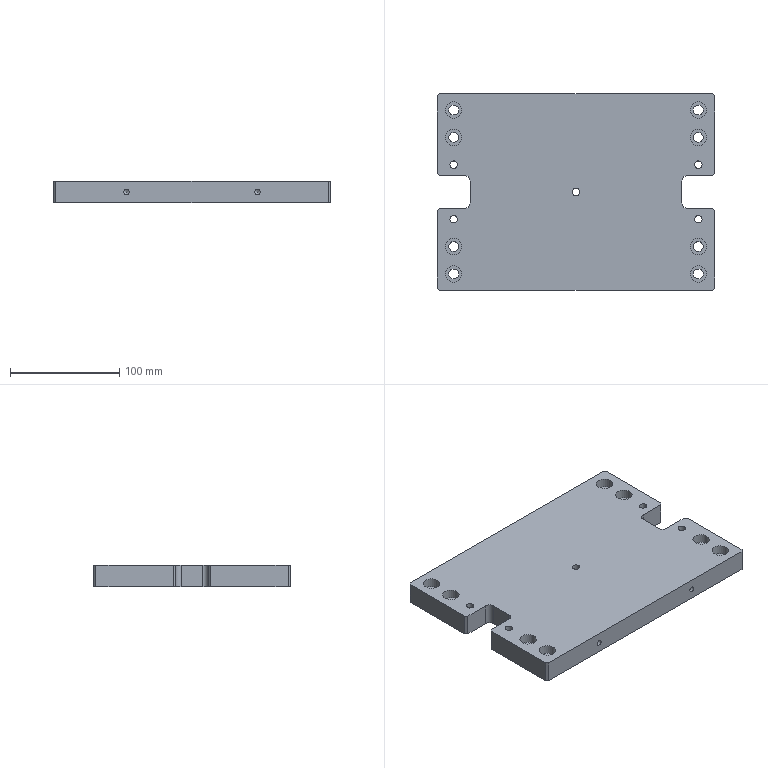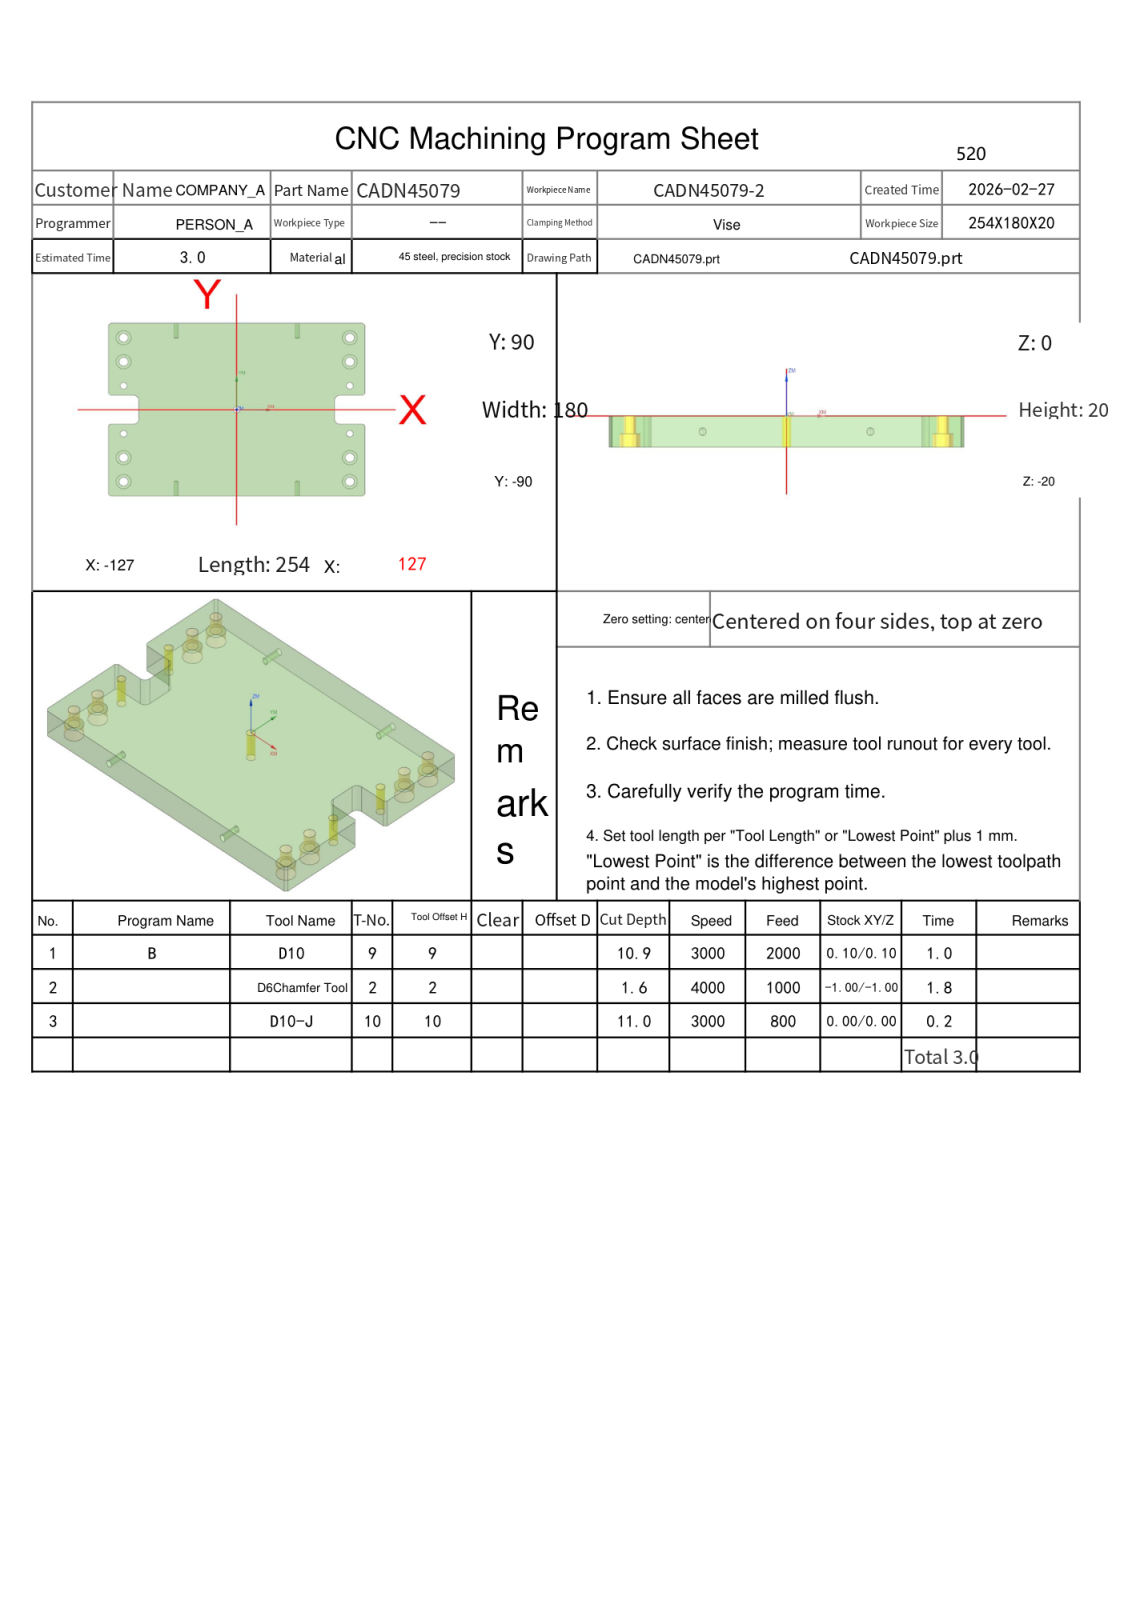NC program | NX | posted by the shop | part box 254 x 180 x 20 mm
Whole program:
%
O0001
(Machine time: 3.55 MIN)
(===Total Tool:3===)
(T9=D10     D=10.  R=0.   D-  H09 Z=-10.9 )
(T2=D6Chamfer Tool   D=6.   R=0.   D-  H02 Z=-1.6  )
(T10=D10-J  D=10.  R=0.   D-  H10 Z=-11.  )
G80 G90 G17 G49 G40
G91 G28 Z0
M01
N1 T09 M06
(D10  D=10. R=0. H=09 ce=0.10 di=0.10)
G00 G90 G54 X122.242 Y99.97 M03 S3000
G43 H09 Z30.
M08
Z-.5
G01 X128.606 Y93.606 F2000.
X130.606 Y91.606
X136.97 Y85.242
G00 Z-1.
G01 X130.606 Y91.606
X128.606 Y93.606
X122.242 Y99.97
G00 Z-1.5
G01 X128.606 Y93.606
X130.606 Y91.606
X136.97 Y85.242
G00 Z-2.
G01 X130.606 Y91.606
X128.606 Y93.606
X122.242 Y99.97
G00 Z-2.5
G01 X128.606 Y93.606
X130.606 Y91.606
X136.97 Y85.242
G00 Z-3.
G01 X130.606 Y91.606
X128.606 Y93.606
X122.242 Y99.97
G00 Z-3.5
G01 X128.606 Y93.606
X130.606 Y91.606
X136.97 Y85.242
G00 Z-4.
G01 X130.606 Y91.606
X128.606 Y93.606
X122.242 Y99.97
G00 Z-4.5
G01 X128.606 Y93.606
X130.606 Y91.606
X136.97 Y85.242
G00 Z-5.
G01 X130.606 Y91.606
X128.606 Y93.606
X122.242 Y99.97
G00 Z-5.5
G01 X128.606 Y93.606
X130.606 Y91.606
X136.97 Y85.242
G00 Z-6.
G01 X130.606 Y91.606
X128.606 Y93.606
X122.242 Y99.97
G00 Z-6.5
G01 X128.606 Y93.606
X130.606 Y91.606
X136.97 Y85.242
G00 Z-7.
G01 X130.606 Y91.606
X128.606 Y93.606
X122.242 Y99.97
G00 Z-7.5
G01 X128.606 Y93.606
X130.606 Y91.606
X136.97 Y85.242
G00 Z-8.
G01 X130.606 Y91.606
X128.606 Y93.606
X122.242 Y99.97
G00 Z-8.5
G01 X128.606 Y93.606
X130.606 Y91.606
X136.97 Y85.242
G00 Z-9.
G01 X130.606 Y91.606
X128.606 Y93.606
X122.242 Y99.97
G00 Z-9.5
G01 X128.606 Y93.606
X130.606 Y91.606
X136.97 Y85.242
G00 Z-10.
G01 X130.606 Y91.606
X128.606 Y93.606
X122.242 Y99.97
G00 Z-10.5
G01 X128.606 Y93.606
X130.606 Y91.606
X136.97 Y85.242
G00 Z-10.9
G01 X130.606 Y91.606
X128.606 Y93.606
X122.242 Y99.97
G00 Z30.
X136.97 Y-85.242
Z-.5
G01 X130.606 Y-91.606
X128.606 Y-93.606
X122.242 Y-99.97
G00 Z-1.
G01 X128.606 Y-93.606
X130.606 Y-91.606
X136.97 Y-85.242
G00 Z-1.5
G01 X130.606 Y-91.606
X128.606 Y-93.606
X122.242 Y-99.97
G00 Z-2.
G01 X128.606 Y-93.606
X130.606 Y-91.606
X136.97 Y-85.242
G00 Z-2.5
G01 X130.606 Y-91.606
X128.606 Y-93.606
X122.242 Y-99.97
G00 Z-3.
G01 X128.606 Y-93.606
X130.606 Y-91.606
X136.97 Y-85.242
G00 Z-3.5
G01 X130.606 Y-91.606
X128.606 Y-93.606
X122.242 Y-99.97
G00 Z-4.
G01 X128.606 Y-93.606
X130.606 Y-91.606
X136.97 Y-85.242
G00 Z-4.5
G01 X130.606 Y-91.606
X128.606 Y-93.606
X122.242 Y-99.97
G00 Z-5.
G01 X128.606 Y-93.606
X130.606 Y-91.606
X136.97 Y-85.242
G00 Z-5.5
G01 X130.606 Y-91.606
X128.606 Y-93.606
X122.242 Y-99.97
G00 Z-6.
G01 X128.606 Y-93.606
X130.606 Y-91.606
X136.97 Y-85.242
G00 Z-6.5
G01 X130.606 Y-91.606
X128.606 Y-93.606
X122.242 Y-99.97
G00 Z-7.
G01 X128.606 Y-93.606
X130.606 Y-91.606
X136.97 Y-85.242
G00 Z-7.5
G01 X130.606 Y-91.606
X128.606 Y-93.606
X122.242 Y-99.97
G00 Z-8.
G01 X128.606 Y-93.606
X130.606 Y-91.606
X136.97 Y-85.242
G00 Z-8.5
G01 X130.606 Y-91.606
X128.606 Y-93.606
X122.242 Y-99.97
G00 Z-9.
G01 X128.606 Y-93.606
X130.606 Y-91.606
X136.97 Y-85.242
G00 Z-9.5
G01 X130.606 Y-91.606
X128.606 Y-93.606
X122.242 Y-99.97
G00 Z-10.
G01 X128.606 Y-93.606
X130.606 Y-91.606
X136.97 Y-85.242
G00 Z-10.5
G01 X130.606 Y-91.606
X128.606 Y-93.606
X122.242 Y-99.97
G00 Z-10.9
G01 X128.606 Y-93.606
X130.606 Y-91.606
X136.97 Y-85.242
G00 Z30.
X-122.242 Y-99.97
Z-.5
G01 X-128.606 Y-93.606
X-130.606 Y-91.606
X-136.97 Y-85.242
G00 Z-1.
G01 X-130.606 Y-91.606
X-128.606 Y-93.606
X-122.242 Y-99.97
G00 Z-1.5
G01 X-128.606 Y-93.606
X-130.606 Y-91.606
X-136.97 Y-85.242
G00 Z-2.
G01 X-130.606 Y-91.606
X-128.606 Y-93.606
X-122.242 Y-99.97
G00 Z-2.5
G01 X-128.606 Y-93.606
X-130.606 Y-91.606
X-136.97 Y-85.242
G00 Z-3.
G01 X-130.606 Y-91.606
X-128.606 Y-93.606
X-122.242 Y-99.97
G00 Z-3.5
G01 X-128.606 Y-93.606
X-130.606 Y-91.606
X-136.97 Y-85.242
G00 Z-4.
G01 X-130.606 Y-91.606
X-128.606 Y-93.606
X-122.242 Y-99.97
G00 Z-4.5
G01 X-128.606 Y-93.606
X-130.606 Y-91.606
X-136.97 Y-85.242
G00 Z-5.
G01 X-130.606 Y-91.606
X-128.606 Y-93.606
X-122.242 Y-99.97
G00 Z-5.5
G01 X-128.606 Y-93.606
X-130.606 Y-91.606
X-136.97 Y-85.242
G00 Z-6.
G01 X-130.606 Y-91.606
X-128.606 Y-93.606
X-122.242 Y-99.97
G00 Z-6.5
G01 X-128.606 Y-93.606
X-130.606 Y-91.606
X-136.97 Y-85.242
G00 Z-7.
G01 X-130.606 Y-91.606
X-128.606 Y-93.606
X-122.242 Y-99.97
G00 Z-7.5
G01 X-128.606 Y-93.606
X-130.606 Y-91.606
X-136.97 Y-85.242
G00 Z-8.
G01 X-130.606 Y-91.606
X-128.606 Y-93.606
X-122.242 Y-99.97
G00 Z-8.5
G01 X-128.606 Y-93.606
X-130.606 Y-91.606
X-136.97 Y-85.242
G00 Z-9.
G01 X-130.606 Y-91.606
X-128.606 Y-93.606
X-122.242 Y-99.97
G00 Z-9.5
G01 X-128.606 Y-93.606
X-130.606 Y-91.606
X-136.97 Y-85.242
G00 Z-10.
G01 X-130.606 Y-91.606
X-128.606 Y-93.606
X-122.242 Y-99.97
G00 Z-10.5
G01 X-128.606 Y-93.606
X-130.606 Y-91.606
X-136.97 Y-85.242
G00 Z-10.9
G01 X-130.606 Y-91.606
X-128.606 Y-93.606
X-122.242 Y-99.97
G00 Z30.
X-136.97 Y85.242
Z-.5
G01 X-130.606 Y91.606
X-128.606 Y93.606
X-122.242 Y99.97
G00 Z-1.
G01 X-128.606 Y93.606
X-130.606 Y91.606
X-136.97 Y85.242
G00 Z-1.5
G01 X-130.606 Y91.606
X-128.606 Y93.606
X-122.242 Y99.97
G00 Z-2.
G01 X-128.606 Y93.606
X-130.606 Y91.606
X-136.97 Y85.242
G00 Z-2.5
G01 X-130.606 Y91.606
X-128.606 Y93.606
X-122.242 Y99.97
G00 Z-3.
G01 X-128.606 Y93.606
X-130.606 Y91.606
X-136.97 Y85.242
G00 Z-3.5
G01 X-130.606 Y91.606
X-128.606 Y93.606
X-122.242 Y99.97
G00 Z-4.
G01 X-128.606 Y93.606
X-130.606 Y91.606
X-136.97 Y85.242
G00 Z-4.5
G01 X-130.606 Y91.606
X-128.606 Y93.606
X-122.242 Y99.97
G00 Z-5.
G01 X-128.606 Y93.606
X-130.606 Y91.606
X-136.97 Y85.242
G00 Z-5.5
G01 X-130.606 Y91.606
X-128.606 Y93.606
X-122.242 Y99.97
G00 Z-6.
G01 X-128.606 Y93.606
X-130.606 Y91.606
X-136.97 Y85.242
G00 Z-6.5
G01 X-130.606 Y91.606
X-128.606 Y93.606
X-122.242 Y99.97
G00 Z-7.
G01 X-128.606 Y93.606
X-130.606 Y91.606
X-136.97 Y85.242
G00 Z-7.5
G01 X-130.606 Y91.606
X-128.606 Y93.606
X-122.242 Y99.97
G00 Z-8.
G01 X-128.606 Y93.606
X-130.606 Y91.606
X-136.97 Y85.242
G00 Z-8.5
G01 X-130.606 Y91.606
X-128.606 Y93.606
X-122.242 Y99.97
G00 Z-9.
G01 X-128.606 Y93.606
X-130.606 Y91.606
X-136.97 Y85.242
G00 Z-9.5
G01 X-130.606 Y91.606
X-128.606 Y93.606
X-122.242 Y99.97
G00 Z-10.
G01 X-128.606 Y93.606
X-130.606 Y91.606
X-136.97 Y85.242
G00 Z-10.5
G01 X-130.606 Y91.606
X-128.606 Y93.606
X-122.242 Y99.97
G00 Z-10.9
G01 X-128.606 Y93.606
X-130.606 Y91.606
X-136.97 Y85.242
G00 Z30.
G91 G28 Z0.0
M05
M09
G91 G28 Z0.0
M01
N2 T02 M06
(D6Chamfer Tool  D=6. R=0. H=02 ce=-1.00 di=-0.80)
G00 G90 G54 X111.005 Y26.5 M03 S4000
G43 H02 Z30.
M08
Z-1.1
G01 Z-1.6 F300.
X110.7
G03 X109.2 Y25. I0.0 J-1.5
X112. Y22.2 I2.8 J0.0
X114.8 Y25. I0.0 J2.8
X112. Y27.8 I-2.8 J0.0
X109.2 Y25. I0.0 J-2.8
X110.7 Y23.5 I1.5 J0.0
G01 X111.005
Z-1.1
G00 Z30.
Y-23.5
Z-1.1
G01 Z-1.6
X110.7
G03 X109.2 Y-25. I0.0 J-1.5
X112. Y-27.8 I2.8 J0.0
X114.8 Y-25. I0.0 J2.8
X112. Y-22.2 I-2.8 J0.0
X109.2 Y-25. I0.0 J-2.8
X110.7 Y-26.5 I1.5 J0.0
G01 X111.005
Z-1.1
G00 Z30.
X-.995 Y1.5
Z-1.1
G01 Z-1.6
X-1.3
G03 X-2.8 Y0.0 I0.0 J-1.5
X0.0 Y-2.8 I2.8 J0.0
X2.8 Y0.0 I0.0 J2.8
X0.0 Y2.8 I-2.8 J0.0
X-2.8 Y0.0 I0.0 J-2.8
X-1.3 Y-1.5 I1.5 J0.0
G01 X-.995
Z-1.1
G00 Z30.
X-112.995 Y-23.5
Z-1.1
G01 Z-1.6
X-113.3
G03 X-114.8 Y-25. I0.0 J-1.5
X-112. Y-27.8 I2.8 J0.0
X-109.2 Y-25. I0.0 J2.8
X-112. Y-22.2 I-2.8 J0.0
X-114.8 Y-25. I0.0 J-2.8
X-113.3 Y-26.5 I1.5 J0.0
G01 X-112.995
Z-1.1
G00 Z30.
Y26.5
Z-1.1
G01 Z-1.6
X-113.3
G03 X-114.8 Y25. I0.0 J-1.5
X-112. Y22.2 I2.8 J0.0
X-109.2 Y25. I0.0 J2.8
X-112. Y27.8 I-2.8 J0.0
X-114.8 Y25. I0.0 J-2.8
X-113.3 Y23.5 I1.5 J0.0
G01 X-112.995
Z-1.1
G00 Z30.
G00 G90 X-.386 Y91.227 M03 S3500
Z30.
Z.172
G01 Z-1.2 F1000.
G03 X-.1 Y91.027 I1.286 J1.532
G01 X-.054 Y90.997
X0.0 Y91.
X125.
X125.259 Y90.966
X125.5 Y90.866
X125.707 Y90.707
X127.707 Y88.707
X127.866 Y88.5
X127.966 Y88.259
X128. Y88.
Y17.
X127.966 Y16.741
X127.866 Y16.5
X127.707 Y16.293
X125.707 Y14.293
X125.5 Y14.134
X125.259 Y14.034
X125. Y14.
X102.
G03 X98. Y10. I0.0 J-4.
G01 Y-10.
G03 X102. Y-14. I4. J0.0
G01 X125.
X125.259 Y-14.034
X125.5 Y-14.134
X125.707 Y-14.293
X127.707 Y-16.293
X127.866 Y-16.5
X127.966 Y-16.741
X128. Y-17.
Y-88.
X127.966 Y-88.259
X127.866 Y-88.5
X127.707 Y-88.707
X125.707 Y-90.707
X125.5 Y-90.866
X125.259 Y-90.966
X125. Y-91.
X-125.
X-125.259 Y-90.966
X-125.5 Y-90.866
X-125.707 Y-90.707
X-127.707 Y-88.707
X-127.866 Y-88.5
X-127.966 Y-88.259
X-128. Y-88.
Y-17.
X-127.966 Y-16.741
X-127.866 Y-16.5
X-127.707 Y-16.293
X-125.707 Y-14.293
X-125.5 Y-14.134
X-125.259 Y-14.034
X-125. Y-14.
X-102.
G03 X-98. Y-10. I0.0 J4.
G01 Y10.
G03 X-102. Y14. I-4. J0.0
G01 X-125.
X-125.259 Y14.034
X-125.5 Y14.134
X-125.707 Y14.293
X-127.707 Y16.293
X-127.866 Y16.5
X-127.966 Y16.741
X-128. Y17.
Y88.
X-127.966 Y88.259
X-127.866 Y88.5
X-127.707 Y88.707
X-125.707 Y90.707
X-125.5 Y90.866
X-125.259 Y90.966
X-125. Y91.
X0.0
X.054 Y90.997
X.1 Y91.027
G03 X.386 Y91.227 I-1. J1.732
G01 Z.172
G00 Z10.
X108.697 Y75.401
Z.23
G01 Z-1.2
G03 X108.519 Y75.102 I1.624 J-1.167
G01 X108.493 Y75.054
X108.5 Y75.
G03 X112. Y71.5 I3.5 J0.0
X115.5 Y75. I0.0 J3.5
X112. Y78.5 I-3.5 J0.0
X108.5 Y75. I0.0 J-3.5
G01 X108.493 Y74.946
X108.519 Y74.898
G03 X108.697 Y74.599 I1.802 J.868
G01 Z.23
G00 Z10.
Y50.401
Z.23
G01 Z-1.2
G03 X108.519 Y50.102 I1.624 J-1.167
G01 X108.493 Y50.054
X108.5 Y50.
G03 X112. Y46.5 I3.5 J0.0
X115.5 Y50. I0.0 J3.5
X112. Y53.5 I-3.5 J0.0
X108.5 Y50. I0.0 J-3.5
G01 X108.493 Y49.946
X108.519 Y49.898
G03 X108.697 Y49.599 I1.802 J.868
G01 Z.23
G00 Z10.
X109.792 Y25.404
Z.252
G01 Z-1.2
G03 X109.618 Y25.102 I1.638 J-1.147
G01 X109.592 Y25.054
X109.6 Y25.
G03 X112. Y22.6 I2.4 J0.0
X114.4 Y25. I0.0 J2.4
X112. Y27.4 I-2.4 J0.0
X109.6 Y25. I0.0 J-2.4
G01 X109.592 Y24.946
X109.618 Y24.898
G03 X109.792 Y24.596 I1.813 J.845
G01 Z.252
G00 Z10.
Y-24.596
Z.252
G01 Z-1.2
G03 X109.618 Y-24.898 I1.638 J-1.147
G01 X109.592 Y-24.946
X109.6 Y-25.
G03 X112. Y-27.4 I2.4 J0.0
X114.4 Y-25. I0.0 J2.4
X112. Y-22.6 I-2.4 J0.0
X109.6 Y-25. I0.0 J-2.4
G01 X109.592 Y-25.054
X109.618 Y-25.102
G03 X109.792 Y-25.404 I1.813 J.845
G01 Z.252
G00 Z10.
X108.697 Y-49.599
Z.23
G01 Z-1.2
G03 X108.519 Y-49.898 I1.624 J-1.167
G01 X108.493 Y-49.946
X108.5 Y-50.
G03 X112. Y-53.5 I3.5 J0.0
X115.5 Y-50. I0.0 J3.5
X112. Y-46.5 I-3.5 J0.0
X108.5 Y-50. I0.0 J-3.5
G01 X108.493 Y-50.054
X108.519 Y-50.102
G03 X108.697 Y-50.401 I1.802 J.868
G01 Z.23
G00 Z10.
Y-74.599
Z.23
G01 Z-1.2
G03 X108.519 Y-74.898 I1.624 J-1.167
G01 X108.493 Y-74.946
X108.5 Y-75.
G03 X112. Y-78.5 I3.5 J0.0
X115.5 Y-75. I0.0 J3.5
X112. Y-71.5 I-3.5 J0.0
X108.5 Y-75. I0.0 J-3.5
G01 X108.493 Y-75.054
X108.519 Y-75.102
G03 X108.697 Y-75.401 I1.802 J.868
G01 Z.23
G00 Z10.
X-2.208 Y.404
Z.252
G01 Z-1.2
G03 X-2.382 Y.102 I1.638 J-1.147
G01 X-2.408 Y.054
X-2.4 Y0.0
G03 X0.0 Y-2.4 I2.4 J0.0
X2.4 Y0.0 I0.0 J2.4
X0.0 Y2.4 I-2.4 J0.0
X-2.4 Y0.0 I0.0 J-2.4
G01 X-2.408 Y-.054
X-2.382 Y-.102
G03 X-2.208 Y-.404 I1.813 J.845
G01 Z.252
G00 Z10.
X-115.303 Y75.401
Z.23
G01 Z-1.2
G03 X-115.481 Y75.102 I1.624 J-1.167
G01 X-115.507 Y75.054
X-115.5 Y75.
G03 X-112. Y71.5 I3.5 J0.0
X-108.5 Y75. I0.0 J3.5
X-112. Y78.5 I-3.5 J0.0
X-115.5 Y75. I0.0 J-3.5
G01 X-115.507 Y74.946
X-115.481 Y74.898
G03 X-115.303 Y74.599 I1.802 J.868
G01 Z.23
G00 Z10.
Y50.401
Z.23
G01 Z-1.2
G03 X-115.481 Y50.102 I1.624 J-1.167
G01 X-115.507 Y50.054
X-115.5 Y50.
G03 X-112. Y46.5 I3.5 J0.0
X-108.5 Y50. I0.0 J3.5
X-112. Y53.5 I-3.5 J0.0
X-115.5 Y50. I0.0 J-3.5
G01 X-115.507 Y49.946
X-115.481 Y49.898
G03 X-115.303 Y49.599 I1.802 J.868
G01 Z.23
G00 Z10.
X-114.208 Y25.404
Z.252
G01 Z-1.2
G03 X-114.382 Y25.102 I1.638 J-1.147
G01 X-114.408 Y25.054
X-114.4 Y25.
G03 X-112. Y22.6 I2.4 J0.0
X-109.6 Y25. I0.0 J2.4
X-112. Y27.4 I-2.4 J0.0
X-114.4 Y25. I0.0 J-2.4
G01 X-114.408 Y24.946
X-114.382 Y24.898
G03 X-114.208 Y24.596 I1.813 J.845
G01 Z.252
G00 Z10.
Y-24.596
Z.252
G01 Z-1.2
G03 X-114.382 Y-24.898 I1.638 J-1.147
G01 X-114.408 Y-24.946
X-114.4 Y-25.
G03 X-112. Y-27.4 I2.4 J0.0
X-109.6 Y-25. I0.0 J2.4
X-112. Y-22.6 I-2.4 J0.0
X-114.4 Y-25. I0.0 J-2.4
G01 X-114.408 Y-25.054
X-114.382 Y-25.102
G03 X-114.208 Y-25.404 I1.813 J.845
G01 Z.252
G00 Z10.
X-115.303 Y-49.599
Z.23
G01 Z-1.2
G03 X-115.481 Y-49.898 I1.624 J-1.167
G01 X-115.507 Y-49.946
X-115.5 Y-50.
G03 X-112. Y-53.5 I3.5 J0.0
X-108.5 Y-50. I0.0 J3.5
X-112. Y-46.5 I-3.5 J0.0
X-115.5 Y-50. I0.0 J-3.5
G01 X-115.507 Y-50.054
X-115.481 Y-50.102
G03 X-115.303 Y-50.401 I1.802 J.868
G01 Z.23
G00 Z10.
Y-74.599
Z.23
G01 Z-1.2
G03 X-115.481 Y-74.898 I1.624 J-1.167
G01 X-115.507 Y-74.946
X-115.5 Y-75.
G03 X-112. Y-78.5 I3.5 J0.0
X-108.5 Y-75. I0.0 J3.5
X-112. Y-71.5 I-3.5 J0.0
X-115.5 Y-75. I0.0 J-3.5
G01 X-115.507 Y-75.054
X-115.481 Y-75.102
G03 X-115.303 Y-75.401 I1.802 J.868
G01 Z.23
G00 Z30.
G91 G28 Z0.0
M05
M09
G91 G28 Z0.0
M01
N3 T10 M06
(D10-J  D=10. R=0. H=10 ce=0.00 di=0.00)
G00 G90 G54 X-124.293 Y-97.778 M03 S3000
G43 H10 Z30.
M08
Z-10.
G01 Z-11. F800.
X-128.536 Y-93.536
X-130.536 Y-91.536
X-134.778 Y-87.293
Z-10.
G00 Z30.
Y87.293
Z-10.
G01 Z-11.
X-130.536 Y91.536
X-128.536 Y93.536
X-124.293 Y97.778
Z-10.
G00 Z30.
X124.293
Z-10.
G01 Z-11.
X128.536 Y93.536
X130.536 Y91.536
X134.778 Y87.293
Z-10.
G00 Z30.
Y-87.293
Z-10.
G01 Z-11.
X130.536 Y-91.536
X128.536 Y-93.536
X124.293 Y-97.778
Z-10.
G00 Z30.
M05
M09
G91 G28 Z0.0
G91 G28 Y0.0
M30
%